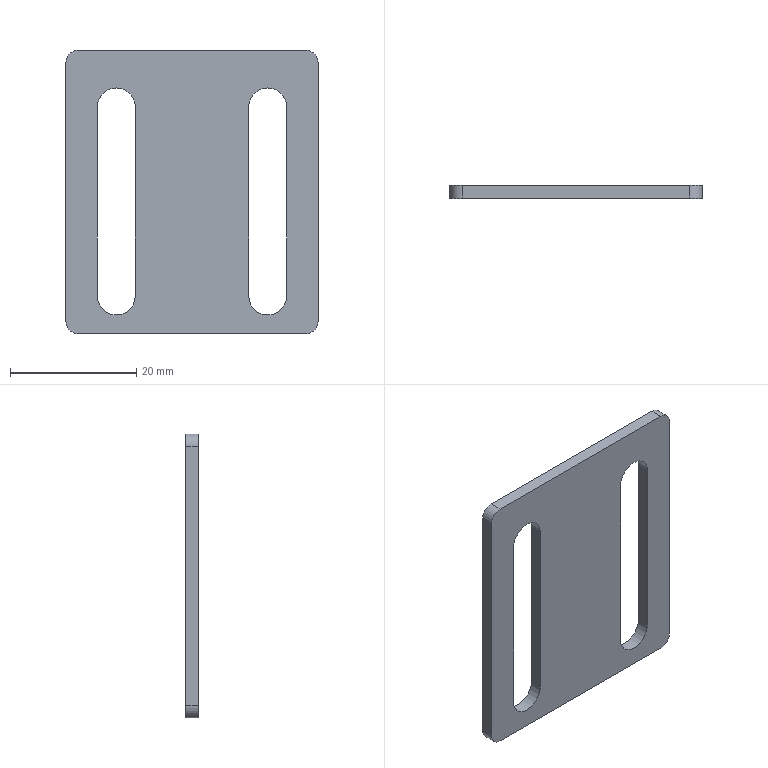Part | STEP file | Clamp plate | 1 solid | 20 faces | box 40 x 2 x 45 mm | volume 2760 mm3 | cylinder 10 | plane 10 | commonest cylinder face diameters 6 x6 4 x4